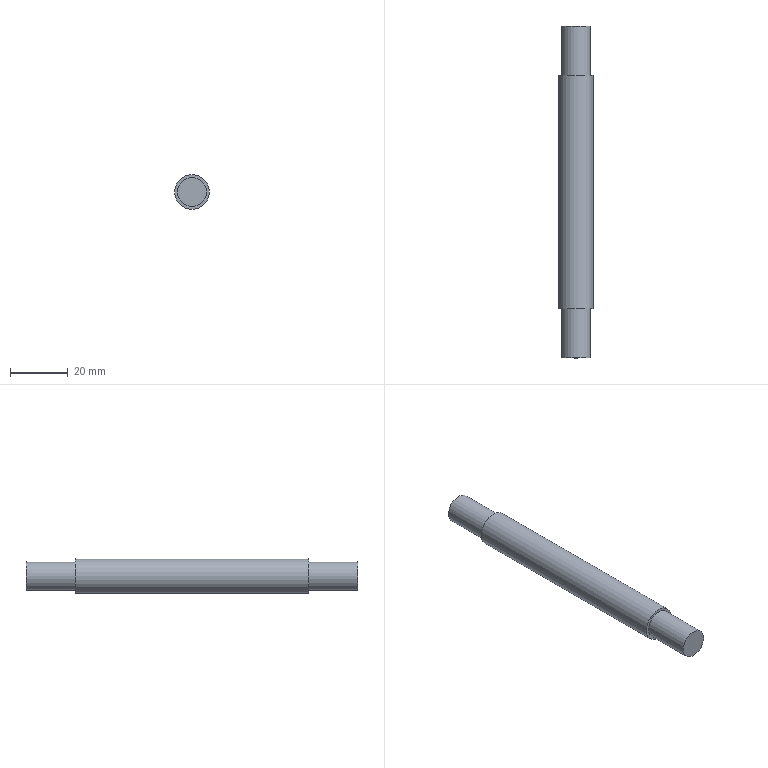Part | STEP file | 2-01.2 | 1 solid | 7 faces | box 12 x 115 x 12 mm | volume 11831 mm3 | plane 4 | cylinder 3 | commonest cylinder face diameters 10 x2 12 x1
STEP:
#1=CARTESIAN_POINT('',(0.,0.,0.));
#2=DIRECTION('',(0.,0.,1.));
#3=DIRECTION('',(1.,0.,0.));
#4=AXIS2_PLACEMENT_3D('',#1,#2,#3);
#5=CARTESIAN_POINT('',(6.,-40.5,0.));
#6=VERTEX_POINT('',#5);
#7=CARTESIAN_POINT('',(6.,40.5,0.));
#8=VERTEX_POINT('',#7);
#9=CARTESIAN_POINT('',(6.,-40.5,0.));
#10=DIRECTION('',(0.,1.,0.));
#11=VECTOR('',#10,1.);
#12=LINE('',#9,#11);
#13=CARTESIAN_POINT('',(0.,-40.5,0.));
#14=DIRECTION('',(0.,1.,0.));
#15=DIRECTION('',(1.,0.,0.));
#16=AXIS2_PLACEMENT_3D('',#13,#14,#15);
#17=CYLINDRICAL_SURFACE('',#16,6.);
#18=CARTESIAN_POINT('',(6.283,0.));
#19=DIRECTION('',(0.,1.));
#20=VECTOR('',#19,1.);
#21=LINE('',#18,#20);
#22=(GEOMETRIC_REPRESENTATION_CONTEXT(2)PARAMETRIC_REPRESENTATION_CONTEXT()REPRESENTATION_CONTEXT('',''));
#23=DEFINITIONAL_REPRESENTATION('',(#21),#22);
#24=PCURVE('',#17,#23);
#25=CARTESIAN_POINT('',(0.,0.));
#26=DIRECTION('',(0.,1.));
#27=VECTOR('',#26,1.);
#28=LINE('',#25,#27);
#29=(GEOMETRIC_REPRESENTATION_CONTEXT(2)PARAMETRIC_REPRESENTATION_CONTEXT()REPRESENTATION_CONTEXT('',''));
#30=DEFINITIONAL_REPRESENTATION('',(#28),#29);
#31=PCURVE('',#17,#30);
#32=SEAM_CURVE('',#12,(#24,#31),.PCURVE_S1.);
#33=EDGE_CURVE('',#6,#8,#32,.T.);
#34=ORIENTED_EDGE('',*,*,#33,.T.);
#35=CARTESIAN_POINT('',(0.,40.5,0.));
#36=DIRECTION('',(0.,-1.,0.));
#37=DIRECTION('',(1.,0.,0.));
#38=AXIS2_PLACEMENT_3D('',#35,#36,#37);
#39=CIRCLE('',#38,6.);
#40=CARTESIAN_POINT('',(6.283,81.));
#41=DIRECTION('',(-1.,0.));
#42=VECTOR('',#41,1.);
#43=LINE('',#40,#42);
#44=(GEOMETRIC_REPRESENTATION_CONTEXT(2)PARAMETRIC_REPRESENTATION_CONTEXT()REPRESENTATION_CONTEXT('',''));
#45=DEFINITIONAL_REPRESENTATION('',(#43),#44);
#46=PCURVE('',#17,#45);
#47=CARTESIAN_POINT('',(-1.608,40.5,0.));
#48=DIRECTION('',(0.,-1.,0.));
#49=DIRECTION('',(1.,0.,0.));
#50=AXIS2_PLACEMENT_3D('',#47,#48,#49);
#51=PLANE('',#50);
#52=CARTESIAN_POINT('',(1.608,0.));
#53=DIRECTION('',(1.,0.));
#54=AXIS2_PLACEMENT_2D('',#52,#53);
#55=CIRCLE('',#54,6.);
#56=(GEOMETRIC_REPRESENTATION_CONTEXT(2)PARAMETRIC_REPRESENTATION_CONTEXT()REPRESENTATION_CONTEXT('',''));
#57=DEFINITIONAL_REPRESENTATION('',(#55),#56);
#58=PCURVE('',#51,#57);
#59=SURFACE_CURVE('',#39,(#46,#58),.PCURVE_S1.);
#60=EDGE_CURVE('',#8,#8,#59,.T.);
#61=ORIENTED_EDGE('',*,*,#60,.T.);
#62=ORIENTED_EDGE('',*,*,#33,.F.);
#63=CARTESIAN_POINT('',(0.,-40.5,0.));
#64=DIRECTION('',(0.,-1.,0.));
#65=DIRECTION('',(1.,0.,0.));
#66=AXIS2_PLACEMENT_3D('',#63,#64,#65);
#67=CIRCLE('',#66,6.);
#68=CARTESIAN_POINT('',(6.283,0.));
#69=DIRECTION('',(-1.,0.));
#70=VECTOR('',#69,1.);
#71=LINE('',#68,#70);
#72=(GEOMETRIC_REPRESENTATION_CONTEXT(2)PARAMETRIC_REPRESENTATION_CONTEXT()REPRESENTATION_CONTEXT('',''));
#73=DEFINITIONAL_REPRESENTATION('',(#71),#72);
#74=PCURVE('',#17,#73);
#75=CARTESIAN_POINT('',(-1.608,-40.5,0.));
#76=DIRECTION('',(0.,-1.,0.));
#77=DIRECTION('',(1.,0.,0.));
#78=AXIS2_PLACEMENT_3D('',#75,#76,#77);
#79=PLANE('',#78);
#80=CARTESIAN_POINT('',(1.608,0.));
#81=DIRECTION('',(1.,0.));
#82=AXIS2_PLACEMENT_2D('',#80,#81);
#83=CIRCLE('',#82,6.);
#84=(GEOMETRIC_REPRESENTATION_CONTEXT(2)PARAMETRIC_REPRESENTATION_CONTEXT()REPRESENTATION_CONTEXT('',''));
#85=DEFINITIONAL_REPRESENTATION('',(#83),#84);
#86=PCURVE('',#79,#85);
#87=SURFACE_CURVE('',#67,(#74,#86),.PCURVE_S1.);
#88=EDGE_CURVE('',#6,#6,#87,.T.);
#89=ORIENTED_EDGE('',*,*,#88,.F.);
#90=EDGE_LOOP('',(#34,#61,#62,#89));
#91=FACE_BOUND('',#90,.T.);
#92=ADVANCED_FACE('',(#91),#17,.T.);
#93=ORIENTED_EDGE('',*,*,#88,.T.);
#94=EDGE_LOOP('',(#93));
#95=FACE_BOUND('',#94,.T.);
#96=CARTESIAN_POINT('',(5.,-40.5,0.));
#97=VERTEX_POINT('',#96);
#98=CARTESIAN_POINT('',(0.,-40.5,0.));
#99=DIRECTION('',(0.,-1.,0.));
#100=DIRECTION('',(1.,0.,0.));
#101=AXIS2_PLACEMENT_3D('',#98,#99,#100);
#102=CIRCLE('',#101,5.);
#103=CARTESIAN_POINT('',(1.608,0.));
#104=DIRECTION('',(1.,0.));
#105=AXIS2_PLACEMENT_2D('',#103,#104);
#106=CIRCLE('',#105,5.);
#107=(GEOMETRIC_REPRESENTATION_CONTEXT(2)PARAMETRIC_REPRESENTATION_CONTEXT()REPRESENTATION_CONTEXT('',''));
#108=DEFINITIONAL_REPRESENTATION('',(#106),#107);
#109=PCURVE('',#79,#108);
#110=CARTESIAN_POINT('',(0.,-40.5,0.));
#111=DIRECTION('',(0.,-1.,0.));
#112=DIRECTION('',(1.,0.,0.));
#113=AXIS2_PLACEMENT_3D('',#110,#111,#112);
#114=CYLINDRICAL_SURFACE('',#113,5.);
#115=CARTESIAN_POINT('',(0.,0.));
#116=DIRECTION('',(1.,0.));
#117=VECTOR('',#116,1.);
#118=LINE('',#115,#117);
#119=(GEOMETRIC_REPRESENTATION_CONTEXT(2)PARAMETRIC_REPRESENTATION_CONTEXT()REPRESENTATION_CONTEXT('',''));
#120=DEFINITIONAL_REPRESENTATION('',(#118),#119);
#121=PCURVE('',#114,#120);
#122=SURFACE_CURVE('',#102,(#109,#121),.PCURVE_S1.);
#123=EDGE_CURVE('',#97,#97,#122,.T.);
#124=ORIENTED_EDGE('',*,*,#123,.F.);
#125=EDGE_LOOP('',(#124));
#126=FACE_BOUND('',#125,.T.);
#127=ADVANCED_FACE('',(#95,#126),#79,.T.);
#128=ORIENTED_EDGE('',*,*,#123,.T.);
#129=CARTESIAN_POINT('',(5.,-57.5,0.));
#130=VERTEX_POINT('',#129);
#131=CARTESIAN_POINT('',(5.,-40.5,0.));
#132=DIRECTION('',(0.,-1.,0.));
#133=VECTOR('',#132,1.);
#134=LINE('',#131,#133);
#135=CARTESIAN_POINT('',(6.283,0.));
#136=DIRECTION('',(0.,1.));
#137=VECTOR('',#136,1.);
#138=LINE('',#135,#137);
#139=(GEOMETRIC_REPRESENTATION_CONTEXT(2)PARAMETRIC_REPRESENTATION_CONTEXT()REPRESENTATION_CONTEXT('',''));
#140=DEFINITIONAL_REPRESENTATION('',(#138),#139);
#141=PCURVE('',#114,#140);
#142=CARTESIAN_POINT('',(0.,0.));
#143=DIRECTION('',(0.,1.));
#144=VECTOR('',#143,1.);
#145=LINE('',#142,#144);
#146=(GEOMETRIC_REPRESENTATION_CONTEXT(2)PARAMETRIC_REPRESENTATION_CONTEXT()REPRESENTATION_CONTEXT('',''));
#147=DEFINITIONAL_REPRESENTATION('',(#145),#146);
#148=PCURVE('',#114,#147);
#149=SEAM_CURVE('',#134,(#141,#148),.PCURVE_S1.);
#150=EDGE_CURVE('',#97,#130,#149,.T.);
#151=ORIENTED_EDGE('',*,*,#150,.T.);
#152=CARTESIAN_POINT('',(0.,-57.5,0.));
#153=DIRECTION('',(0.,-1.,0.));
#154=DIRECTION('',(1.,0.,0.));
#155=AXIS2_PLACEMENT_3D('',#152,#153,#154);
#156=CIRCLE('',#155,5.);
#157=CARTESIAN_POINT('',(0.,17.));
#158=DIRECTION('',(1.,0.));
#159=VECTOR('',#158,1.);
#160=LINE('',#157,#159);
#161=(GEOMETRIC_REPRESENTATION_CONTEXT(2)PARAMETRIC_REPRESENTATION_CONTEXT()REPRESENTATION_CONTEXT('',''));
#162=DEFINITIONAL_REPRESENTATION('',(#160),#161);
#163=PCURVE('',#114,#162);
#164=CARTESIAN_POINT('',(-1.34,-57.5,0.));
#165=DIRECTION('',(0.,-1.,0.));
#166=DIRECTION('',(1.,0.,0.));
#167=AXIS2_PLACEMENT_3D('',#164,#165,#166);
#168=PLANE('',#167);
#169=CARTESIAN_POINT('',(1.34,0.));
#170=DIRECTION('',(1.,0.));
#171=AXIS2_PLACEMENT_2D('',#169,#170);
#172=CIRCLE('',#171,5.);
#173=(GEOMETRIC_REPRESENTATION_CONTEXT(2)PARAMETRIC_REPRESENTATION_CONTEXT()REPRESENTATION_CONTEXT('',''));
#174=DEFINITIONAL_REPRESENTATION('',(#172),#173);
#175=PCURVE('',#168,#174);
#176=SURFACE_CURVE('',#156,(#163,#175),.PCURVE_S1.);
#177=EDGE_CURVE('',#130,#130,#176,.T.);
#178=ORIENTED_EDGE('',*,*,#177,.F.);
#179=ORIENTED_EDGE('',*,*,#150,.F.);
#180=EDGE_LOOP('',(#128,#151,#178,#179));
#181=FACE_BOUND('',#180,.T.);
#182=ADVANCED_FACE('',(#181),#114,.T.);
#183=ORIENTED_EDGE('',*,*,#177,.T.);
#184=EDGE_LOOP('',(#183));
#185=FACE_BOUND('',#184,.T.);
#186=ADVANCED_FACE('',(#185),#168,.T.);
#187=ORIENTED_EDGE('',*,*,#60,.T.);
#188=EDGE_LOOP('',(#187));
#189=FACE_BOUND('',#188,.F.);
#190=CARTESIAN_POINT('',(5.,40.5,0.));
#191=VERTEX_POINT('',#190);
#192=CARTESIAN_POINT('',(0.,40.5,0.));
#193=DIRECTION('',(0.,-1.,0.));
#194=DIRECTION('',(1.,0.,0.));
#195=AXIS2_PLACEMENT_3D('',#192,#193,#194);
#196=CIRCLE('',#195,5.);
#197=CARTESIAN_POINT('',(1.608,0.));
#198=DIRECTION('',(1.,0.));
#199=AXIS2_PLACEMENT_2D('',#197,#198);
#200=CIRCLE('',#199,5.);
#201=(GEOMETRIC_REPRESENTATION_CONTEXT(2)PARAMETRIC_REPRESENTATION_CONTEXT()REPRESENTATION_CONTEXT('',''));
#202=DEFINITIONAL_REPRESENTATION('',(#200),#201);
#203=PCURVE('',#51,#202);
#204=CARTESIAN_POINT('',(0.,40.5,0.));
#205=DIRECTION('',(0.,1.,0.));
#206=DIRECTION('',(1.,0.,0.));
#207=AXIS2_PLACEMENT_3D('',#204,#205,#206);
#208=CYLINDRICAL_SURFACE('',#207,5.);
#209=CARTESIAN_POINT('',(6.283,0.));
#210=DIRECTION('',(-1.,0.));
#211=VECTOR('',#210,1.);
#212=LINE('',#209,#211);
#213=(GEOMETRIC_REPRESENTATION_CONTEXT(2)PARAMETRIC_REPRESENTATION_CONTEXT()REPRESENTATION_CONTEXT('',''));
#214=DEFINITIONAL_REPRESENTATION('',(#212),#213);
#215=PCURVE('',#208,#214);
#216=SURFACE_CURVE('',#196,(#203,#215),.PCURVE_S1.);
#217=EDGE_CURVE('',#191,#191,#216,.T.);
#218=ORIENTED_EDGE('',*,*,#217,.F.);
#219=EDGE_LOOP('',(#218));
#220=FACE_BOUND('',#219,.F.);
#221=ADVANCED_FACE('',(#189,#220),#51,.F.);
#222=CARTESIAN_POINT('',(5.,57.5,0.));
#223=VERTEX_POINT('',#222);
#224=CARTESIAN_POINT('',(5.,40.5,0.));
#225=DIRECTION('',(0.,1.,0.));
#226=VECTOR('',#225,1.);
#227=LINE('',#224,#226);
#228=CARTESIAN_POINT('',(6.283,0.));
#229=DIRECTION('',(0.,1.));
#230=VECTOR('',#229,1.);
#231=LINE('',#228,#230);
#232=(GEOMETRIC_REPRESENTATION_CONTEXT(2)PARAMETRIC_REPRESENTATION_CONTEXT()REPRESENTATION_CONTEXT('',''));
#233=DEFINITIONAL_REPRESENTATION('',(#231),#232);
#234=PCURVE('',#208,#233);
#235=CARTESIAN_POINT('',(0.,0.));
#236=DIRECTION('',(0.,1.));
#237=VECTOR('',#236,1.);
#238=LINE('',#235,#237);
#239=(GEOMETRIC_REPRESENTATION_CONTEXT(2)PARAMETRIC_REPRESENTATION_CONTEXT()REPRESENTATION_CONTEXT('',''));
#240=DEFINITIONAL_REPRESENTATION('',(#238),#239);
#241=PCURVE('',#208,#240);
#242=SEAM_CURVE('',#227,(#234,#241),.PCURVE_S1.);
#243=EDGE_CURVE('',#191,#223,#242,.T.);
#244=ORIENTED_EDGE('',*,*,#243,.T.);
#245=CARTESIAN_POINT('',(0.,57.5,0.));
#246=DIRECTION('',(0.,-1.,0.));
#247=DIRECTION('',(1.,0.,0.));
#248=AXIS2_PLACEMENT_3D('',#245,#246,#247);
#249=CIRCLE('',#248,5.);
#250=CARTESIAN_POINT('',(6.283,17.));
#251=DIRECTION('',(-1.,0.));
#252=VECTOR('',#251,1.);
#253=LINE('',#250,#252);
#254=(GEOMETRIC_REPRESENTATION_CONTEXT(2)PARAMETRIC_REPRESENTATION_CONTEXT()REPRESENTATION_CONTEXT('',''));
#255=DEFINITIONAL_REPRESENTATION('',(#253),#254);
#256=PCURVE('',#208,#255);
#257=CARTESIAN_POINT('',(-1.34,57.5,0.));
#258=DIRECTION('',(0.,-1.,0.));
#259=DIRECTION('',(1.,0.,0.));
#260=AXIS2_PLACEMENT_3D('',#257,#258,#259);
#261=PLANE('',#260);
#262=CARTESIAN_POINT('',(1.34,0.));
#263=DIRECTION('',(1.,0.));
#264=AXIS2_PLACEMENT_2D('',#262,#263);
#265=CIRCLE('',#264,5.);
#266=(GEOMETRIC_REPRESENTATION_CONTEXT(2)PARAMETRIC_REPRESENTATION_CONTEXT()REPRESENTATION_CONTEXT('',''));
#267=DEFINITIONAL_REPRESENTATION('',(#265),#266);
#268=PCURVE('',#261,#267);
#269=SURFACE_CURVE('',#249,(#256,#268),.PCURVE_S1.);
#270=EDGE_CURVE('',#223,#223,#269,.T.);
#271=ORIENTED_EDGE('',*,*,#270,.T.);
#272=ORIENTED_EDGE('',*,*,#243,.F.);
#273=ORIENTED_EDGE('',*,*,#217,.F.);
#274=EDGE_LOOP('',(#244,#271,#272,#273));
#275=FACE_BOUND('',#274,.T.);
#276=ADVANCED_FACE('',(#275),#208,.T.);
#277=ORIENTED_EDGE('',*,*,#270,.T.);
#278=EDGE_LOOP('',(#277));
#279=FACE_BOUND('',#278,.F.);
#280=ADVANCED_FACE('',(#279),#261,.F.);
#281=CLOSED_SHELL('',(#92,#127,#182,#186,#221,#276,#280));
#282=MANIFOLD_SOLID_BREP('',#281);
#283=(LENGTH_UNIT()NAMED_UNIT(*)SI_UNIT(.MILLI.,.METRE.));
#284=UNCERTAINTY_MEASURE_WITH_UNIT(LENGTH_MEASURE(0.0000001),#283,'','');
#285=(NAMED_UNIT(*)PLANE_ANGLE_UNIT()SI_UNIT($,.RADIAN.));
#286=(NAMED_UNIT(*)SI_UNIT($,.STERADIAN.)SOLID_ANGLE_UNIT());
#287=(GEOMETRIC_REPRESENTATION_CONTEXT(3)GLOBAL_UNCERTAINTY_ASSIGNED_CONTEXT((#284))GLOBAL_UNIT_ASSIGNED_CONTEXT((#283,#285,#286))REPRESENTATION_CONTEXT('',''));
#288=ADVANCED_BREP_SHAPE_REPRESENTATION('',(#4,#282),#287);